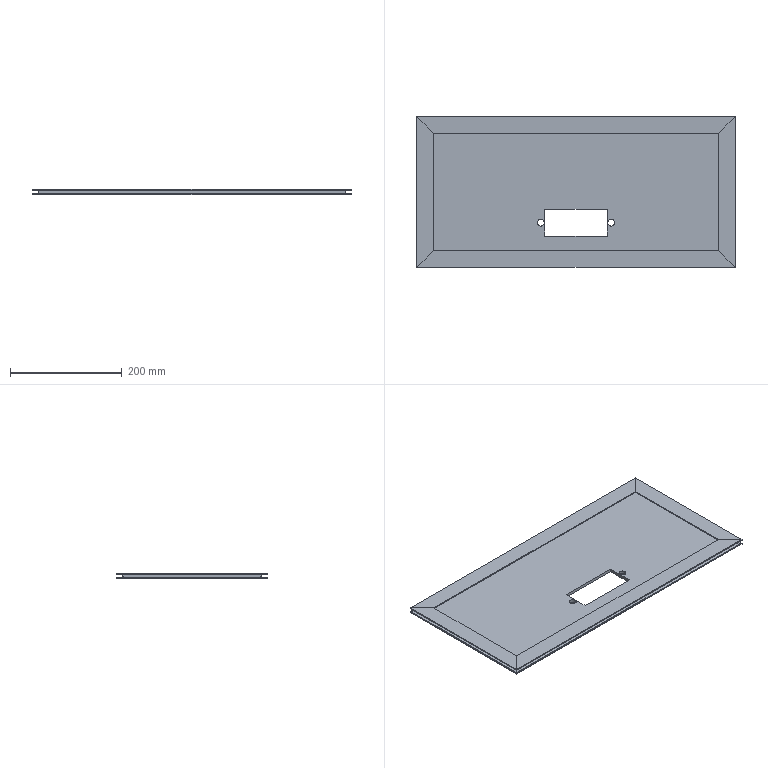Part | SolidWorks | features ICE 2, WeldMemberFeat 1, WeldmentFeature 1 | 5 solids | 102 faces | box 570 x 270 x 10 mm | volume 810104 mm3 | plane 82 | cylinder 20 | commonest cylinder face diameters 2 x16 12 x4